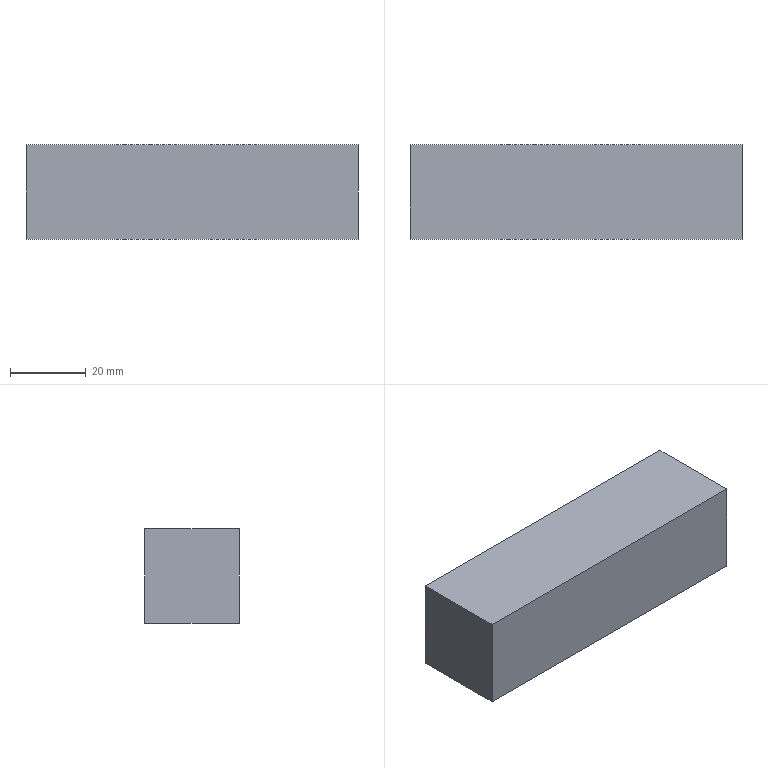Part | NX | features solid 2 | 1 solid | 6 faces | box 87.841 x 25 x 25 mm | volume 54901 mm3 | plane 6
STEP:
#1=CARTESIAN_POINT('',(570.,305.,35.));
#2=VERTEX_POINT('',#1);
#3=CARTESIAN_POINT('',(570.,280.,35.));
#4=VERTEX_POINT('',#3);
#5=CARTESIAN_POINT('',(570.,305.,35.));
#6=DIRECTION('',(0.,1.,0.));
#7=VECTOR('',#6,1000.);
#8=LINE('',#5,#7);
#9=EDGE_CURVE('',#2,#4,#8,.F.);
#10=ORIENTED_EDGE('',*,*,#9,.T.);
#11=CARTESIAN_POINT('',(657.841,280.,35.));
#12=VERTEX_POINT('',#11);
#13=CARTESIAN_POINT('',(672.841,280.,35.));
#14=DIRECTION('',(1.,0.,0.));
#15=VECTOR('',#14,1000.);
#16=LINE('',#13,#15);
#17=EDGE_CURVE('',#12,#4,#16,.F.);
#18=ORIENTED_EDGE('',*,*,#17,.F.);
#19=CARTESIAN_POINT('',(657.841,305.,35.));
#20=VERTEX_POINT('',#19);
#21=CARTESIAN_POINT('',(657.841,305.,35.));
#22=DIRECTION('',(0.,-1.,0.));
#23=VECTOR('',#22,1000.);
#24=LINE('',#21,#23);
#25=EDGE_CURVE('',#20,#12,#24,.T.);
#26=ORIENTED_EDGE('',*,*,#25,.F.);
#27=CARTESIAN_POINT('',(672.841,305.,35.));
#28=DIRECTION('',(1.,0.,0.));
#29=VECTOR('',#28,1000.);
#30=LINE('',#27,#29);
#31=EDGE_CURVE('',#20,#2,#30,.F.);
#32=ORIENTED_EDGE('',*,*,#31,.T.);
#33=EDGE_LOOP('',(#10,#18,#26,#32));
#34=FACE_BOUND('',#33,.T.);
#35=CARTESIAN_POINT('',(672.841,305.,35.));
#36=DIRECTION('',(0.,0.,-1.));
#37=DIRECTION('',(-1.,0.,0.));
#38=AXIS2_PLACEMENT_3D('',#35,#36,#37);
#39=PLANE('',#38);
#40=ADVANCED_FACE('',(#34),#39,.F.);
#41=CARTESIAN_POINT('',(657.841,305.,10.));
#42=VERTEX_POINT('',#41);
#43=CARTESIAN_POINT('',(657.841,305.,-30.));
#44=DIRECTION('',(0.,0.,-1.));
#45=VECTOR('',#44,1000.);
#46=LINE('',#43,#45);
#47=EDGE_CURVE('',#42,#20,#46,.F.);
#48=ORIENTED_EDGE('',*,*,#47,.F.);
#49=CARTESIAN_POINT('',(570.,305.,10.));
#50=VERTEX_POINT('',#49);
#51=CARTESIAN_POINT('',(672.841,305.,10.));
#52=DIRECTION('',(-1.,0.,0.));
#53=VECTOR('',#52,1000.);
#54=LINE('',#51,#53);
#55=EDGE_CURVE('',#42,#50,#54,.T.);
#56=ORIENTED_EDGE('',*,*,#55,.T.);
#57=CARTESIAN_POINT('',(570.,305.,-30.));
#58=DIRECTION('',(0.,0.,1.));
#59=VECTOR('',#58,1000.);
#60=LINE('',#57,#59);
#61=EDGE_CURVE('',#50,#2,#60,.T.);
#62=ORIENTED_EDGE('',*,*,#61,.T.);
#63=ORIENTED_EDGE('',*,*,#31,.F.);
#64=EDGE_LOOP('',(#48,#56,#62,#63));
#65=FACE_BOUND('',#64,.T.);
#66=CARTESIAN_POINT('',(672.841,305.,-30.));
#67=DIRECTION('',(0.,-1.,0.));
#68=DIRECTION('',(0.,0.,-1.));
#69=AXIS2_PLACEMENT_3D('',#66,#67,#68);
#70=PLANE('',#69);
#71=ADVANCED_FACE('',(#65),#70,.F.);
#72=CARTESIAN_POINT('',(657.841,280.,10.));
#73=VERTEX_POINT('',#72);
#74=CARTESIAN_POINT('',(657.841,-320.,10.));
#75=DIRECTION('',(0.,1.,0.));
#76=VECTOR('',#75,1000.);
#77=LINE('',#74,#76);
#78=EDGE_CURVE('',#73,#42,#77,.T.);
#79=ORIENTED_EDGE('',*,*,#78,.T.);
#80=ORIENTED_EDGE('',*,*,#47,.T.);
#81=ORIENTED_EDGE('',*,*,#25,.T.);
#82=CARTESIAN_POINT('',(657.841,280.,-30.));
#83=DIRECTION('',(0.,0.,-1.));
#84=VECTOR('',#83,1000.);
#85=LINE('',#82,#84);
#86=EDGE_CURVE('',#73,#12,#85,.F.);
#87=ORIENTED_EDGE('',*,*,#86,.F.);
#88=EDGE_LOOP('',(#79,#80,#81,#87));
#89=FACE_BOUND('',#88,.T.);
#90=CARTESIAN_POINT('',(657.841,305.,-30.));
#91=DIRECTION('',(-1.,0.,0.));
#92=DIRECTION('',(0.,0.,1.));
#93=AXIS2_PLACEMENT_3D('',#90,#91,#92);
#94=PLANE('',#93);
#95=ADVANCED_FACE('',(#89),#94,.F.);
#96=ORIENTED_EDGE('',*,*,#61,.F.);
#97=CARTESIAN_POINT('',(570.,280.,10.));
#98=VERTEX_POINT('',#97);
#99=CARTESIAN_POINT('',(570.,-320.,10.));
#100=DIRECTION('',(0.,1.,0.));
#101=VECTOR('',#100,1000.);
#102=LINE('',#99,#101);
#103=EDGE_CURVE('',#50,#98,#102,.F.);
#104=ORIENTED_EDGE('',*,*,#103,.T.);
#105=CARTESIAN_POINT('',(570.,280.,-30.));
#106=DIRECTION('',(0.,0.,1.));
#107=VECTOR('',#106,1000.);
#108=LINE('',#105,#107);
#109=EDGE_CURVE('',#98,#4,#108,.T.);
#110=ORIENTED_EDGE('',*,*,#109,.T.);
#111=ORIENTED_EDGE('',*,*,#9,.F.);
#112=EDGE_LOOP('',(#96,#104,#110,#111));
#113=FACE_BOUND('',#112,.T.);
#114=CARTESIAN_POINT('',(570.,305.,-30.));
#115=DIRECTION('',(-1.,0.,0.));
#116=DIRECTION('',(0.,0.,1.));
#117=AXIS2_PLACEMENT_3D('',#114,#115,#116);
#118=PLANE('',#117);
#119=ADVANCED_FACE('',(#113),#118,.T.);
#120=ORIENTED_EDGE('',*,*,#109,.F.);
#121=CARTESIAN_POINT('',(940.,280.,10.));
#122=DIRECTION('',(-1.,0.,0.));
#123=VECTOR('',#122,1000.);
#124=LINE('',#121,#123);
#125=EDGE_CURVE('',#98,#73,#124,.F.);
#126=ORIENTED_EDGE('',*,*,#125,.T.);
#127=ORIENTED_EDGE('',*,*,#86,.T.);
#128=ORIENTED_EDGE('',*,*,#17,.T.);
#129=EDGE_LOOP('',(#120,#126,#127,#128));
#130=FACE_BOUND('',#129,.T.);
#131=CARTESIAN_POINT('',(672.841,280.,-30.));
#132=DIRECTION('',(0.,-1.,0.));
#133=DIRECTION('',(0.,0.,-1.));
#134=AXIS2_PLACEMENT_3D('',#131,#132,#133);
#135=PLANE('',#134);
#136=ADVANCED_FACE('',(#130),#135,.T.);
#137=ORIENTED_EDGE('',*,*,#78,.F.);
#138=ORIENTED_EDGE('',*,*,#125,.F.);
#139=ORIENTED_EDGE('',*,*,#103,.F.);
#140=ORIENTED_EDGE('',*,*,#55,.F.);
#141=EDGE_LOOP('',(#137,#138,#139,#140));
#142=FACE_BOUND('',#141,.T.);
#143=CARTESIAN_POINT('',(-202.,435.,10.));
#144=DIRECTION('',(0.,0.,1.));
#145=DIRECTION('',(1.,0.,0.));
#146=AXIS2_PLACEMENT_3D('',#143,#144,#145);
#147=PLANE('',#146);
#148=ADVANCED_FACE('',(#142),#147,.F.);
#149=CLOSED_SHELL('',(#40,#71,#95,#119,#136,#148));
#150=MANIFOLD_SOLID_BREP('',#149);
#151=(LENGTH_UNIT()NAMED_UNIT(*)SI_UNIT(.MILLI.,.METRE.));
#152=UNCERTAINTY_MEASURE_WITH_UNIT(LENGTH_MEASURE(0.00001),#151,'','');
#153=(NAMED_UNIT(*)PLANE_ANGLE_UNIT()SI_UNIT($,.RADIAN.));
#154=(NAMED_UNIT(*)SI_UNIT($,.STERADIAN.)SOLID_ANGLE_UNIT());
#155=(GEOMETRIC_REPRESENTATION_CONTEXT(3)GLOBAL_UNCERTAINTY_ASSIGNED_CONTEXT((#152))GLOBAL_UNIT_ASSIGNED_CONTEXT((#151,#153,#154))REPRESENTATION_CONTEXT('',''));
#156=ADVANCED_BREP_SHAPE_REPRESENTATION('',(#150),#155);